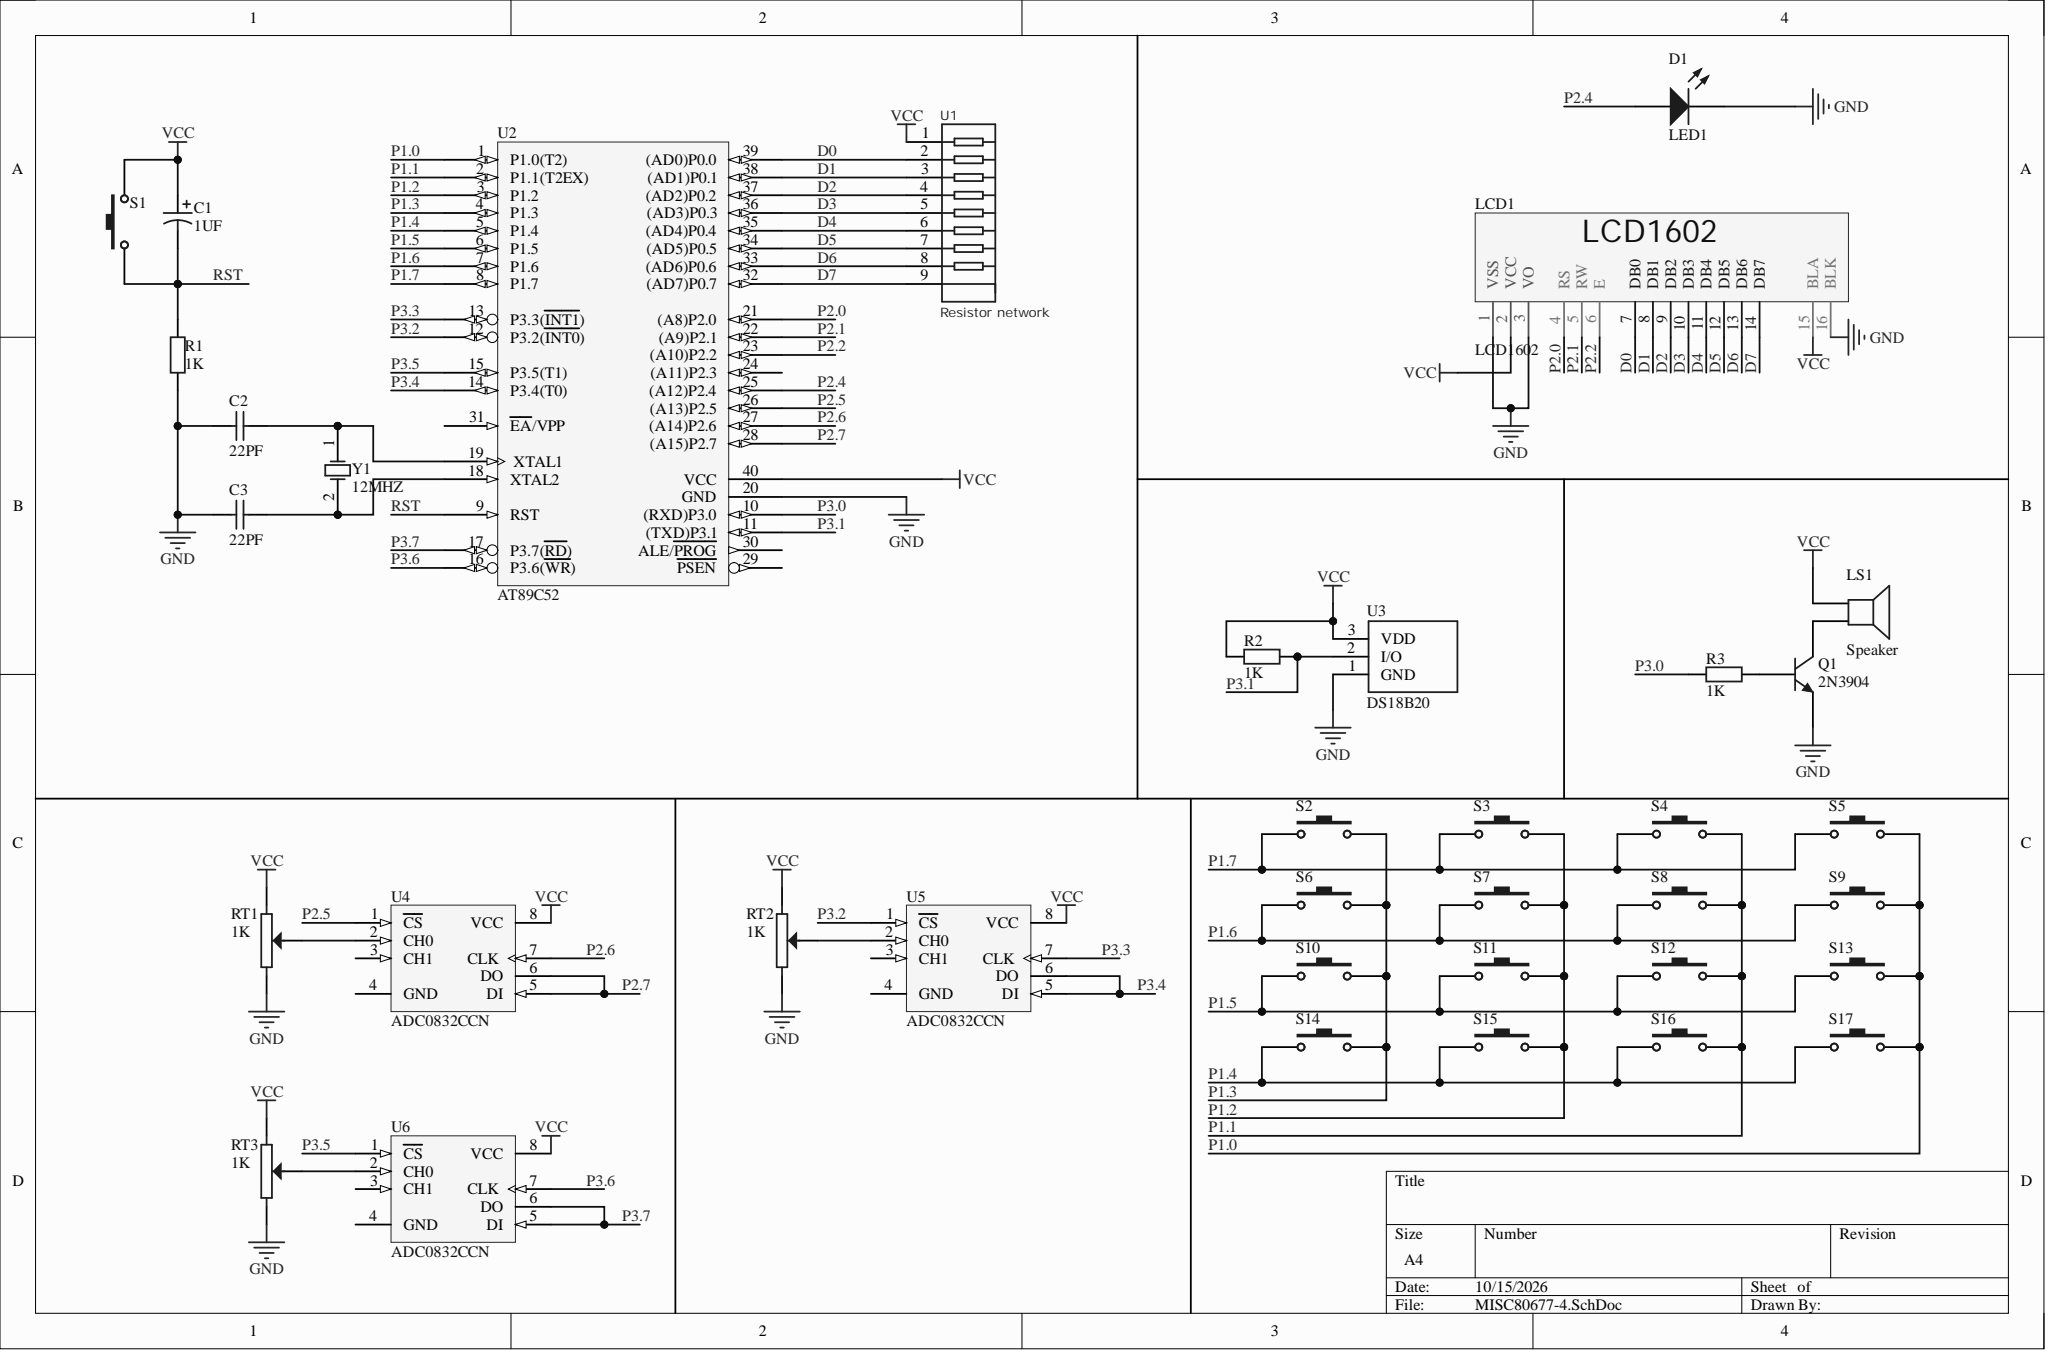Circuit board | Altium Designer | 37 parts | 41 nets
Bill of materials:
Comment,Description,Designator,Footprint,LibRef,Quantity
"1UF","Polarized Capacitor (Radial)","C1","RB7.6-15","Cap Pol1","1"
"22PF","Capacitor","C2, C3","RAD-0.3","Cap","2"
"LED1","Typical RED GaAs LED","D1","LED-1","LED1","1"
"LCD1602","","LCD1","LCD1602","LCD1602","1"
"Speaker","Loudspeaker","LS1","PIN2","Speaker","1"
"2N3904","NPN General Purpose Amplifier","Q1","TO-92A","2N3904","1"
"1K","Resistor","R1, R2, R3","AXIAL-0.4","Res2","3"
"1K","","RT1, RT2, RT3","电位器","电位器","3"
"SW-PB","Switch","S1, S2, S3, S4, S5, S6, S7, S8, S9, S10, S11, S12, S13, S14, S15, S16, S17","SPST-2","SW-PB","17"
"Resistor network","","U1","paizu","排阻","1"
"AT89C52","","U2","DIP40","STC89C52","1"
"DS18B20","","U3","DS18B20","DS18B20","1"
"ADC0832CCN","8-Bit Serial I/O A/D Converter with Multiplexer Option","U4, U5, U6","N08E","ADC0832CCN","3"
"12MHZ","Crystal Oscillator","Y1","R38","XTAL","1"
Netlist (Protel format):
[
C1
RB7.6-15
1UF



]
[
C2
RAD-0.3
22PF



]
[
C3
RAD-0.3
22PF



]
[
D1
LED-1
LED1



]
[
LCD1
LCD1602
LCD1602



]
[
LS1
PIN2
Speaker



]
[
Q1
TO-92A
2N3904



]
[
R1
AXIAL-0.4
1K



]
[
R2
AXIAL-0.4
1K



]
[
R3
AXIAL-0.4
1K



]
[
RT1
电位器
1K



]
[
RT2
电位器
1K



]
[
RT3
电位器
1K



]
[
S1
SPST-2
SW-PB



]
[
S2
SPST-2
SW-PB



]
[
S3
SPST-2
SW-PB



]
[
S4
SPST-2
SW-PB



]
[
S5
SPST-2
SW-PB



]
[
S6
SPST-2
SW-PB



]
[
S7
SPST-2
SW-PB



]
[
S8
SPST-2
SW-PB



]
[
S9
SPST-2
SW-PB



]
[
S10
SPST-2
SW-PB



]
[
S11
SPST-2
SW-PB



]
[
S12
SPST-2
SW-PB



]
[
S13
SPST-2
SW-PB



]
[
S14
SPST-2
SW-PB



]
[
S15
SPST-2
SW-PB



]
[
S16
SPST-2
SW-PB



]
[
S17
SPST-2
SW-PB



]
[
U1
paizu
Resistor network



]
[
U2
DIP40
AT89C52



]
[
U3
DS18B20
DS18B20



]
[
U4
N08E
ADC0832CCN



]
[
U5
N08E
ADC0832CCN



]
[
U6
N08E
ADC0832CCN



]
[
Y1
R38
12MHZ



]
(
VCC
C1-1
LCD1-2
LCD1-15
LS1-1
R2-1
RT1-1
RT2-1
RT3-1
S1-2
U1-1
U2-40
U3-3
U4-8
U5-8
U6-8
)
(
RST
C1-2
R1-2
S1-1
U2-9
)
(
P3.7
U2-17
U6-5
U6-6
)
(
P3.6
U2-16
U6-7
)
(
P3.5
U2-15
U6-1
)
(
P3.4
U2-14
U5-5
U5-6
)
(
P3.3
U2-13
U5-7
)
(
P3.2
U2-12
U5-1
)
(
P3.1
R2-2
U2-11
U3-2
)
(
P3.0
R3-1
U2-10
)
(
P2.7
U2-28
U4-5
U4-6
)
(
P2.6
U2-27
U4-7
)
(
P2.5
U2-26
U4-1
)
(
P2.4
D1-1
U2-25
)
(
P2.2
LCD1-6
U2-23
)
(
P2.1
LCD1-5
U2-22
)
(
P2.0
LCD1-4
U2-21
)
(
P1.7
S2-1
S3-1
S4-1
S5-1
U2-8
)
(
P1.6
S6-1
S7-1
S8-1
S9-1
U2-7
)
(
P1.5
S10-1
S11-1
S12-1
S13-1
U2-6
)
(
P1.4
S14-1
S15-1
S16-1
S17-1
U2-5
)
(
P1.3
S2-2
S6-2
S10-2
S14-2
U2-4
)
(
P1.2
S3-2
S7-2
S11-2
S15-2
U2-3
)
(
P1.1
S4-2
S8-2
S12-2
S16-2
U2-2
)
(
P1.0
S5-2
S9-2
S13-2
S17-2
U2-1
)
(
NetRT3_3
RT3-3
U6-2
)
(
NetRT2_3
RT2-3
U5-2
)
(
NetRT1_3
RT1-3
U4-2
)
(
NetQ1_2
Q1-2
R3-2
)
(
NetLS1_2
LS1-2
Q1-3
)
(
NetC3_2
C3-2
U2-18
Y1-2
)
(
NetC2_2
C2-2
U2-19
Y1-1
)
(
GND
C2-1
C3-1
D1-2
LCD1-1
LCD1-3
LCD1-16
Q1-1
R1-1
RT1-2
RT2-2
RT3-2
U2-20
U3-1
)
(
D7
LCD1-14
U1-9
U2-32
)
(
D6
LCD1-13
U1-8
U2-33
)
(
D5
LCD1-12
U1-7
U2-34
)
(
D4
LCD1-11
U1-6
U2-35
)
(
D3
LCD1-10
U1-5
U2-36
)
(
D2
LCD1-9
U1-4
U2-37
)
(
D1
LCD1-8
U1-3
U2-38
)
(
D0
LCD1-7
U1-2
U2-39
)